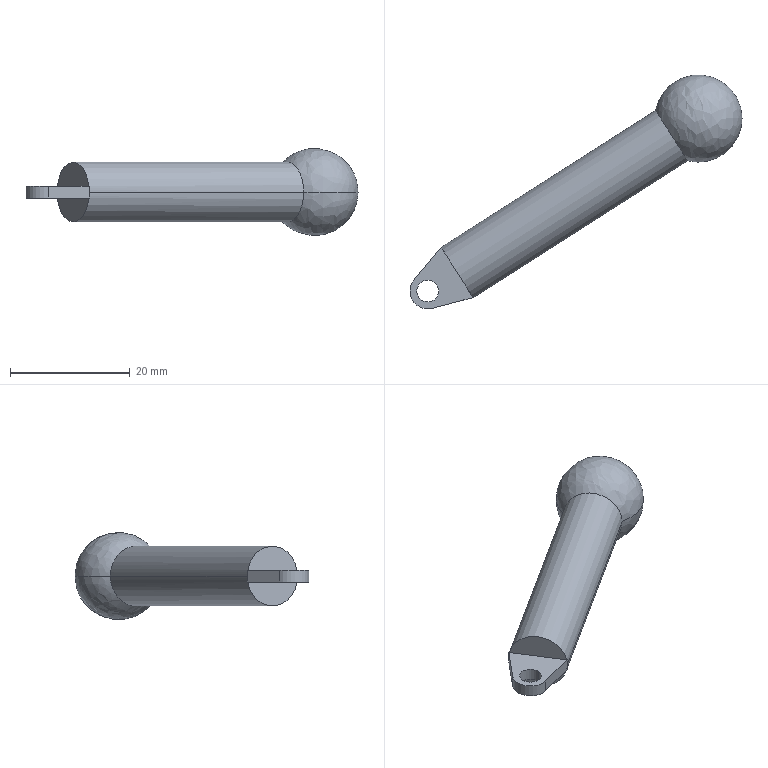Part | SolidWorks | features BaseBody 1 | 1 solid | 17 faces | box 55.474 x 39.094 x 14.478 mm | volume 4963 mm3 | plane 10 | cylinder 5 | spline 2 | commonest cylinder face diameters 3.663 x2 9.977 x2 5.943 x1
STEP:
#1=CARTESIAN_POINT('',(-130.74,-10.361,0.));
#2=VERTEX_POINT('',#1);
#3=CARTESIAN_POINT('',(-145.183,-9.009,0.));
#4=VERTEX_POINT('',#3);
#5=CARTESIAN_POINT('',(-138.024,-10.361,0.));
#6=DIRECTION('',(0.,0.,1.));
#7=DIRECTION('',(1.,0.,0.));
#8=AXIS2_PLACEMENT_3D('',#5,#6,#7);
#9=CIRCLE('',#8,7.285);
#10=EDGE_CURVE('',#2,#4,#9,.T.);
#11=ORIENTED_EDGE('',*,*,#10,.F.);
#12=CARTESIAN_POINT('',(-139.818,-17.421,0.));
#13=VERTEX_POINT('',#12);
#14=CARTESIAN_POINT('',(-138.024,-10.361,0.));
#15=DIRECTION('',(0.,0.,-1.));
#16=DIRECTION('',(1.,0.,0.));
#17=AXIS2_PLACEMENT_3D('',#14,#15,#16);
#18=CIRCLE('',#17,7.285);
#19=EDGE_CURVE('',#2,#13,#18,.T.);
#20=ORIENTED_EDGE('',*,*,#19,.T.);
#21=CARTESIAN_POINT('',(-142.5,-13.215,0.));
#22=DIRECTION('',(-0.8431,-0.5377,0.));
#23=DIRECTION('',(-0.5377,0.8431,0.));
#24=AXIS2_PLACEMENT_3D('',#21,#22,#23);
#25=CIRCLE('',#24,4.989);
#26=EDGE_CURVE('',#4,#13,#25,.T.);
#27=ORIENTED_EDGE('',*,*,#26,.F.);
#28=EDGE_LOOP('',(#11,#20,#27));
#29=FACE_OUTER_BOUND('',#28,.T.);
#30=CARTESIAN_POINT('',(-130.74,-10.361,0.));
#31=CARTESIAN_POINT('',(-130.74,-10.361,0.));
#32=CARTESIAN_POINT('',(-130.74,-10.361,0.));
#33=CARTESIAN_POINT('',(-130.74,-10.361,0.));
#34=CARTESIAN_POINT('',(-130.74,-22.783,0.));
#35=CARTESIAN_POINT('',(-130.74,-22.783,-24.844));
#36=CARTESIAN_POINT('',(-130.74,2.061,-24.844));
#37=CARTESIAN_POINT('',(-130.74,2.061,0.));
#38=CARTESIAN_POINT('',(-143.118,-23.83,0.));
#39=CARTESIAN_POINT('',(-143.118,-23.83,-26.94));
#40=CARTESIAN_POINT('',(-143.118,3.109,-26.94));
#41=CARTESIAN_POINT('',(-143.118,3.109,0.));
#42=CARTESIAN_POINT('',(-145.205,-11.585,0.));
#43=CARTESIAN_POINT('',(-145.205,-11.585,-2.449));
#44=CARTESIAN_POINT('',(-145.205,-9.136,-2.449));
#45=CARTESIAN_POINT('',(-145.205,-9.136,0.));
#46=(BOUNDED_SURFACE()B_SPLINE_SURFACE(3,3,((#30,#31,#32,#33),(#34,#35,#36,#37),(#38,#39,#40,#41),(#42,#43,#44,#45)),.UNSPECIFIED.,.F.,.F.,.F.)B_SPLINE_SURFACE_WITH_KNOTS((4,4),(4,4),(0.,1.),(0.,1.),.UNSPECIFIED.)GEOMETRIC_REPRESENTATION_ITEM()RATIONAL_B_SPLINE_SURFACE(((1.,0.3333,0.3333,1.),(0.3896,0.1299,0.1299,0.3896),(0.3896,0.1299,0.1299,0.3896),(1.,0.3333,0.3333,1.)))REPRESENTATION_ITEM('')SURFACE());
#47=ADVANCED_FACE('',(#29),#46,.T.);
#48=CARTESIAN_POINT('',(-175.716,-40.195,1.));
#49=VERTEX_POINT('',#48);
#50=CARTESIAN_POINT('',(-175.661,-40.281,0.));
#51=VERTEX_POINT('',#50);
#52=CARTESIAN_POINT('',(-178.344,-36.075,0.));
#53=DIRECTION('',(0.8431,0.5377,0.));
#54=DIRECTION('',(-0.5377,0.8431,0.));
#55=AXIS2_PLACEMENT_3D('',#52,#53,#54);
#56=CIRCLE('',#55,4.989);
#57=EDGE_CURVE('',#49,#51,#56,.T.);
#58=ORIENTED_EDGE('',*,*,#57,.T.);
#59=CARTESIAN_POINT('',(-157.74,-28.851,0.));
#60=DIRECTION('',(0.8431,0.5377,0.));
#61=VECTOR('',#60,1000.);
#62=LINE('',#59,#61);
#63=EDGE_CURVE('',#51,#13,#62,.T.);
#64=ORIENTED_EDGE('',*,*,#63,.T.);
#65=CARTESIAN_POINT('',(-142.5,-13.215,0.));
#66=DIRECTION('',(-0.8431,-0.5377,0.));
#67=DIRECTION('',(-0.5377,0.8431,0.));
#68=AXIS2_PLACEMENT_3D('',#65,#66,#67);
#69=CIRCLE('',#68,4.989);
#70=EDGE_CURVE('',#13,#4,#69,.T.);
#71=ORIENTED_EDGE('',*,*,#70,.T.);
#72=CARTESIAN_POINT('',(-181.026,-31.869,0.));
#73=VERTEX_POINT('',#72);
#74=CARTESIAN_POINT('',(-163.104,-20.439,0.));
#75=DIRECTION('',(0.8431,0.5377,0.));
#76=VECTOR('',#75,1000.);
#77=LINE('',#74,#76);
#78=EDGE_CURVE('',#73,#4,#77,.T.);
#79=ORIENTED_EDGE('',*,*,#78,.F.);
#80=CARTESIAN_POINT('',(-180.972,-31.954,1.));
#81=VERTEX_POINT('',#80);
#82=CARTESIAN_POINT('',(-178.344,-36.075,0.));
#83=DIRECTION('',(0.8431,0.5377,0.));
#84=DIRECTION('',(-0.5377,0.8431,0.));
#85=AXIS2_PLACEMENT_3D('',#82,#83,#84);
#86=CIRCLE('',#85,4.989);
#87=EDGE_CURVE('',#73,#81,#86,.T.);
#88=ORIENTED_EDGE('',*,*,#87,.T.);
#89=CARTESIAN_POINT('',(-178.344,-36.075,0.));
#90=DIRECTION('',(0.8431,0.5377,0.));
#91=DIRECTION('',(-0.5377,0.8431,0.));
#92=AXIS2_PLACEMENT_3D('',#89,#90,#91);
#93=CIRCLE('',#92,4.989);
#94=EDGE_CURVE('',#81,#49,#93,.T.);
#95=ORIENTED_EDGE('',*,*,#94,.T.);
#96=EDGE_LOOP('',(#58,#64,#71,#79,#88,#95));
#97=FACE_OUTER_BOUND('',#96,.T.);
#98=CARTESIAN_POINT('',(-160.422,-24.645,0.));
#99=DIRECTION('',(0.8431,0.5377,0.));
#100=DIRECTION('',(-0.5377,0.8431,0.));
#101=AXIS2_PLACEMENT_3D('',#98,#99,#100);
#102=CYLINDRICAL_SURFACE('',#101,4.989);
#103=ADVANCED_FACE('',(#97),#102,.T.);
#104=CARTESIAN_POINT('',(-181.411,-39.199,-1.));
#105=VERTEX_POINT('',#104);
#106=CARTESIAN_POINT('',(-185.074,-39.199,-1.));
#107=VERTEX_POINT('',#106);
#108=CARTESIAN_POINT('',(-183.243,-39.199,-1.));
#109=DIRECTION('',(0.,0.,-1.));
#110=DIRECTION('',(1.,0.,0.));
#111=AXIS2_PLACEMENT_3D('',#108,#109,#110);
#112=CIRCLE('',#111,1.832);
#113=EDGE_CURVE('',#105,#107,#112,.T.);
#114=ORIENTED_EDGE('',*,*,#113,.T.);
#115=CARTESIAN_POINT('',(-185.074,-39.199,1.));
#116=VERTEX_POINT('',#115);
#117=CARTESIAN_POINT('',(-185.074,-39.199,0.));
#118=DIRECTION('',(0.,0.,1.));
#119=VECTOR('',#118,1000.);
#120=LINE('',#117,#119);
#121=EDGE_CURVE('',#107,#116,#120,.T.);
#122=ORIENTED_EDGE('',*,*,#121,.T.);
#123=CARTESIAN_POINT('',(-181.411,-39.199,1.));
#124=VERTEX_POINT('',#123);
#125=CARTESIAN_POINT('',(-183.243,-39.199,1.));
#126=DIRECTION('',(0.,0.,-1.));
#127=DIRECTION('',(1.,0.,0.));
#128=AXIS2_PLACEMENT_3D('',#125,#126,#127);
#129=CIRCLE('',#128,1.832);
#130=EDGE_CURVE('',#124,#116,#129,.T.);
#131=ORIENTED_EDGE('',*,*,#130,.F.);
#132=CARTESIAN_POINT('',(-181.411,-39.199,0.));
#133=DIRECTION('',(0.,0.,1.));
#134=VECTOR('',#133,1000.);
#135=LINE('',#132,#134);
#136=EDGE_CURVE('',#105,#124,#135,.T.);
#137=ORIENTED_EDGE('',*,*,#136,.F.);
#138=EDGE_LOOP('',(#114,#122,#131,#137));
#139=FACE_OUTER_BOUND('',#138,.T.);
#140=CARTESIAN_POINT('',(-183.243,-39.199,0.));
#141=DIRECTION('',(0.,0.,1.));
#142=DIRECTION('',(1.,0.,0.));
#143=AXIS2_PLACEMENT_3D('',#140,#141,#142);
#144=CYLINDRICAL_SURFACE('',#143,1.832);
#145=ADVANCED_FACE('',(#139),#144,.F.);
#146=ORIENTED_EDGE('',*,*,#63,.F.);
#147=CARTESIAN_POINT('',(-175.716,-40.195,-1.));
#148=VERTEX_POINT('',#147);
#149=CARTESIAN_POINT('',(-178.344,-36.075,0.));
#150=DIRECTION('',(0.8431,0.5377,0.));
#151=DIRECTION('',(-0.5377,0.8431,0.));
#152=AXIS2_PLACEMENT_3D('',#149,#150,#151);
#153=CIRCLE('',#152,4.989);
#154=EDGE_CURVE('',#51,#148,#153,.T.);
#155=ORIENTED_EDGE('',*,*,#154,.T.);
#156=CARTESIAN_POINT('',(-180.972,-31.954,-1.));
#157=VERTEX_POINT('',#156);
#158=CARTESIAN_POINT('',(-178.344,-36.075,0.));
#159=DIRECTION('',(0.8431,0.5377,0.));
#160=DIRECTION('',(-0.5377,0.8431,0.));
#161=AXIS2_PLACEMENT_3D('',#158,#159,#160);
#162=CIRCLE('',#161,4.989);
#163=EDGE_CURVE('',#148,#157,#162,.T.);
#164=ORIENTED_EDGE('',*,*,#163,.T.);
#165=CARTESIAN_POINT('',(-178.344,-36.075,0.));
#166=DIRECTION('',(0.8431,0.5377,0.));
#167=DIRECTION('',(-0.5377,0.8431,0.));
#168=AXIS2_PLACEMENT_3D('',#165,#166,#167);
#169=CIRCLE('',#168,4.989);
#170=EDGE_CURVE('',#157,#73,#169,.T.);
#171=ORIENTED_EDGE('',*,*,#170,.T.);
#172=ORIENTED_EDGE('',*,*,#78,.T.);
#173=ORIENTED_EDGE('',*,*,#26,.T.);
#174=EDGE_LOOP('',(#146,#155,#164,#171,#172,#173));
#175=FACE_OUTER_BOUND('',#174,.T.);
#176=CARTESIAN_POINT('',(-160.422,-24.645,0.));
#177=DIRECTION('',(0.8431,0.5377,0.));
#178=DIRECTION('',(-0.5377,0.8431,0.));
#179=AXIS2_PLACEMENT_3D('',#176,#177,#178);
#180=CYLINDRICAL_SURFACE('',#179,4.989);
#181=ADVANCED_FACE('',(#175),#180,.T.);
#182=ORIENTED_EDGE('',*,*,#19,.F.);
#183=ORIENTED_EDGE('',*,*,#10,.T.);
#184=ORIENTED_EDGE('',*,*,#70,.F.);
#185=EDGE_LOOP('',(#182,#183,#184));
#186=FACE_OUTER_BOUND('',#185,.T.);
#187=CARTESIAN_POINT('',(-130.74,-10.361,0.));
#188=CARTESIAN_POINT('',(-130.74,-10.361,0.));
#189=CARTESIAN_POINT('',(-130.74,-10.361,0.));
#190=CARTESIAN_POINT('',(-130.74,-10.361,0.));
#191=CARTESIAN_POINT('',(-130.74,2.061,0.));
#192=CARTESIAN_POINT('',(-130.74,2.061,24.844));
#193=CARTESIAN_POINT('',(-130.74,-22.783,24.844));
#194=CARTESIAN_POINT('',(-130.74,-22.783,0.));
#195=CARTESIAN_POINT('',(-143.118,3.109,0.));
#196=CARTESIAN_POINT('',(-143.118,3.109,26.94));
#197=CARTESIAN_POINT('',(-143.118,-23.83,26.94));
#198=CARTESIAN_POINT('',(-143.118,-23.83,0.));
#199=CARTESIAN_POINT('',(-145.205,-9.136,0.));
#200=CARTESIAN_POINT('',(-145.205,-9.136,2.449));
#201=CARTESIAN_POINT('',(-145.205,-11.585,2.449));
#202=CARTESIAN_POINT('',(-145.205,-11.585,0.));
#203=(BOUNDED_SURFACE()B_SPLINE_SURFACE(3,3,((#187,#188,#189,#190),(#191,#192,#193,#194),(#195,#196,#197,#198),(#199,#200,#201,#202)),.UNSPECIFIED.,.F.,.F.,.F.)B_SPLINE_SURFACE_WITH_KNOTS((4,4),(4,4),(0.,1.),(0.,1.),.UNSPECIFIED.)GEOMETRIC_REPRESENTATION_ITEM()RATIONAL_B_SPLINE_SURFACE(((1.,0.3333,0.3333,1.),(0.3896,0.1299,0.1299,0.3896),(0.3896,0.1299,0.1299,0.3896),(1.,0.3333,0.3333,1.)))REPRESENTATION_ITEM('')SURFACE());
#204=ADVANCED_FACE('',(#186),#203,.T.);
#205=CARTESIAN_POINT('',(-175.661,-40.281,1.));
#206=VERTEX_POINT('',#205);
#207=CARTESIAN_POINT('',(-175.661,-40.281,1.));
#208=DIRECTION('',(-0.5377,0.8431,0.));
#209=VECTOR('',#208,1000.);
#210=LINE('',#207,#209);
#211=EDGE_CURVE('',#206,#49,#210,.T.);
#212=ORIENTED_EDGE('',*,*,#211,.F.);
#213=CARTESIAN_POINT('',(-175.661,-40.281,0.));
#214=DIRECTION('',(0.,0.,1.));
#215=VECTOR('',#214,1000.);
#216=LINE('',#213,#215);
#217=EDGE_CURVE('',#51,#206,#216,.T.);
#218=ORIENTED_EDGE('',*,*,#217,.F.);
#219=ORIENTED_EDGE('',*,*,#57,.F.);
#220=EDGE_LOOP('',(#212,#218,#219));
#221=FACE_OUTER_BOUND('',#220,.T.);
#222=CARTESIAN_POINT('',(-175.661,-40.281,0.));
#223=DIRECTION('',(0.8431,0.5377,0.));
#224=DIRECTION('',(-0.5377,0.8431,0.));
#225=AXIS2_PLACEMENT_3D('',#222,#223,#224);
#226=PLANE('',#225);
#227=ADVANCED_FACE('',(#221),#226,.T.);
#228=CARTESIAN_POINT('',(-181.026,-31.869,1.));
#229=DIRECTION('',(0.5377,-0.8431,0.));
#230=VECTOR('',#229,1000.);
#231=LINE('',#228,#230);
#232=EDGE_CURVE('',#81,#49,#231,.T.);
#233=ORIENTED_EDGE('',*,*,#232,.T.);
#234=ORIENTED_EDGE('',*,*,#94,.F.);
#235=EDGE_LOOP('',(#233,#234));
#236=FACE_OUTER_BOUND('',#235,.T.);
#237=CARTESIAN_POINT('',(-181.026,-31.869,0.));
#238=DIRECTION('',(-0.8431,-0.5377,0.));
#239=DIRECTION('',(0.5377,-0.8431,0.));
#240=AXIS2_PLACEMENT_3D('',#237,#238,#239);
#241=PLANE('',#240);
#242=ADVANCED_FACE('',(#236),#241,.T.);
#243=CARTESIAN_POINT('',(-181.026,-31.869,1.));
#244=VERTEX_POINT('',#243);
#245=CARTESIAN_POINT('',(-181.026,-31.869,0.));
#246=DIRECTION('',(0.,0.,-1.));
#247=VECTOR('',#246,1000.);
#248=LINE('',#245,#247);
#249=EDGE_CURVE('',#244,#73,#248,.T.);
#250=ORIENTED_EDGE('',*,*,#249,.F.);
#251=CARTESIAN_POINT('',(-175.661,-40.281,1.));
#252=DIRECTION('',(0.5377,-0.8431,0.));
#253=VECTOR('',#252,1000.);
#254=LINE('',#251,#253);
#255=EDGE_CURVE('',#244,#81,#254,.T.);
#256=ORIENTED_EDGE('',*,*,#255,.T.);
#257=ORIENTED_EDGE('',*,*,#87,.F.);
#258=EDGE_LOOP('',(#250,#256,#257));
#259=FACE_OUTER_BOUND('',#258,.T.);
#260=CARTESIAN_POINT('',(-175.661,-40.281,0.));
#261=DIRECTION('',(0.8431,0.5377,0.));
#262=DIRECTION('',(-0.5377,0.8431,0.));
#263=AXIS2_PLACEMENT_3D('',#260,#261,#262);
#264=PLANE('',#263);
#265=ADVANCED_FACE('',(#259),#264,.T.);
#266=CARTESIAN_POINT('',(-181.026,-31.869,-1.));
#267=VERTEX_POINT('',#266);
#268=CARTESIAN_POINT('',(-180.972,-31.954,-1.));
#269=DIRECTION('',(-0.5377,0.8431,0.));
#270=VECTOR('',#269,1000.);
#271=LINE('',#268,#270);
#272=EDGE_CURVE('',#157,#267,#271,.T.);
#273=ORIENTED_EDGE('',*,*,#272,.T.);
#274=CARTESIAN_POINT('',(-181.026,-31.869,0.));
#275=DIRECTION('',(0.,0.,-1.));
#276=VECTOR('',#275,1000.);
#277=LINE('',#274,#276);
#278=EDGE_CURVE('',#73,#267,#277,.T.);
#279=ORIENTED_EDGE('',*,*,#278,.F.);
#280=ORIENTED_EDGE('',*,*,#170,.F.);
#281=EDGE_LOOP('',(#273,#279,#280));
#282=FACE_OUTER_BOUND('',#281,.T.);
#283=CARTESIAN_POINT('',(-175.661,-40.281,0.));
#284=DIRECTION('',(0.8431,0.5377,0.));
#285=DIRECTION('',(-0.5377,0.8431,0.));
#286=AXIS2_PLACEMENT_3D('',#283,#284,#285);
#287=PLANE('',#286);
#288=ADVANCED_FACE('',(#282),#287,.T.);
#289=CARTESIAN_POINT('',(-181.026,-31.869,-1.));
#290=DIRECTION('',(-0.5377,0.8431,0.));
#291=VECTOR('',#290,1000.);
#292=LINE('',#289,#291);
#293=EDGE_CURVE('',#148,#157,#292,.T.);
#294=ORIENTED_EDGE('',*,*,#293,.T.);
#295=ORIENTED_EDGE('',*,*,#163,.F.);
#296=EDGE_LOOP('',(#294,#295));
#297=FACE_OUTER_BOUND('',#296,.T.);
#298=CARTESIAN_POINT('',(-181.026,-31.869,0.));
#299=DIRECTION('',(-0.8431,-0.5377,0.));
#300=DIRECTION('',(0.5377,-0.8431,0.));
#301=AXIS2_PLACEMENT_3D('',#298,#299,#300);
#302=PLANE('',#301);
#303=ADVANCED_FACE('',(#297),#302,.T.);
#304=CARTESIAN_POINT('',(-175.661,-40.281,-1.));
#305=VERTEX_POINT('',#304);
#306=CARTESIAN_POINT('',(-175.661,-40.281,0.));
#307=DIRECTION('',(0.,0.,1.));
#308=VECTOR('',#307,1000.);
#309=LINE('',#306,#308);
#310=EDGE_CURVE('',#305,#51,#309,.T.);
#311=ORIENTED_EDGE('',*,*,#310,.F.);
#312=CARTESIAN_POINT('',(-175.661,-40.281,-1.));
#313=DIRECTION('',(-0.5377,0.8431,0.));
#314=VECTOR('',#313,1000.);
#315=LINE('',#312,#314);
#316=EDGE_CURVE('',#305,#148,#315,.T.);
#317=ORIENTED_EDGE('',*,*,#316,.T.);
#318=ORIENTED_EDGE('',*,*,#154,.F.);
#319=EDGE_LOOP('',(#311,#317,#318));
#320=FACE_OUTER_BOUND('',#319,.T.);
#321=CARTESIAN_POINT('',(-175.661,-40.281,0.));
#322=DIRECTION('',(0.8431,0.5377,0.));
#323=DIRECTION('',(-0.5377,0.8431,0.));
#324=AXIS2_PLACEMENT_3D('',#321,#322,#323);
#325=PLANE('',#324);
#326=ADVANCED_FACE('',(#320),#325,.T.);
#327=ORIENTED_EDGE('',*,*,#130,.T.);
#328=CARTESIAN_POINT('',(-183.243,-39.199,1.));
#329=DIRECTION('',(0.,0.,-1.));
#330=DIRECTION('',(1.,0.,0.));
#331=AXIS2_PLACEMENT_3D('',#328,#329,#330);
#332=CIRCLE('',#331,1.832);
#333=EDGE_CURVE('',#116,#124,#332,.T.);
#334=ORIENTED_EDGE('',*,*,#333,.T.);
#335=EDGE_LOOP('',(#327,#334));
#336=FACE_BOUND('',#335,.T.);
#337=ORIENTED_EDGE('',*,*,#232,.F.);
#338=ORIENTED_EDGE('',*,*,#255,.F.);
#339=CARTESIAN_POINT('',(-185.53,-37.303,1.));
#340=VERTEX_POINT('',#339);
#341=CARTESIAN_POINT('',(-181.026,-31.869,1.));
#342=DIRECTION('',(-0.6382,-0.7699,0.));
#343=VECTOR('',#342,1000.);
#344=LINE('',#341,#343);
#345=EDGE_CURVE('',#244,#340,#344,.T.);
#346=ORIENTED_EDGE('',*,*,#345,.T.);
#347=CARTESIAN_POINT('',(-182.488,-42.073,1.));
#348=VERTEX_POINT('',#347);
#349=CARTESIAN_POINT('',(-183.243,-39.199,1.));
#350=DIRECTION('',(0.,0.,1.));
#351=DIRECTION('',(1.,0.,0.));
#352=AXIS2_PLACEMENT_3D('',#349,#350,#351);
#353=CIRCLE('',#352,2.971);
#354=EDGE_CURVE('',#340,#348,#353,.T.);
#355=ORIENTED_EDGE('',*,*,#354,.T.);
#356=CARTESIAN_POINT('',(-182.488,-42.073,1.));
#357=DIRECTION('',(0.9672,0.2539,0.));
#358=VECTOR('',#357,1000.);
#359=LINE('',#356,#358);
#360=EDGE_CURVE('',#348,#206,#359,.T.);
#361=ORIENTED_EDGE('',*,*,#360,.T.);
#362=ORIENTED_EDGE('',*,*,#211,.T.);
#363=EDGE_LOOP('',(#337,#338,#346,#355,#361,#362));
#364=FACE_OUTER_BOUND('',#363,.T.);
#365=CARTESIAN_POINT('',(-180.938,-37.02,1.));
#366=DIRECTION('',(0.,0.,1.));
#367=DIRECTION('',(1.,0.,0.));
#368=AXIS2_PLACEMENT_3D('',#365,#366,#367);
#369=PLANE('',#368);
#370=ADVANCED_FACE('',(#336,#364),#369,.T.);
#371=ORIENTED_EDGE('',*,*,#113,.F.);
#372=CARTESIAN_POINT('',(-183.243,-39.199,-1.));
#373=DIRECTION('',(0.,0.,-1.));
#374=DIRECTION('',(1.,0.,0.));
#375=AXIS2_PLACEMENT_3D('',#372,#373,#374);
#376=CIRCLE('',#375,1.832);
#377=EDGE_CURVE('',#107,#105,#376,.T.);
#378=ORIENTED_EDGE('',*,*,#377,.F.);
#379=EDGE_LOOP('',(#371,#378));
#380=FACE_BOUND('',#379,.T.);
#381=ORIENTED_EDGE('',*,*,#272,.F.);
#382=ORIENTED_EDGE('',*,*,#293,.F.);
#383=ORIENTED_EDGE('',*,*,#316,.F.);
#384=CARTESIAN_POINT('',(-182.488,-42.073,-1.));
#385=VERTEX_POINT('',#384);
#386=CARTESIAN_POINT('',(-182.488,-42.073,-1.));
#387=DIRECTION('',(0.9672,0.2539,0.));
#388=VECTOR('',#387,1000.);
#389=LINE('',#386,#388);
#390=EDGE_CURVE('',#385,#305,#389,.T.);
#391=ORIENTED_EDGE('',*,*,#390,.F.);
#392=CARTESIAN_POINT('',(-185.53,-37.303,-1.));
#393=VERTEX_POINT('',#392);
#394=CARTESIAN_POINT('',(-183.243,-39.199,-1.));
#395=DIRECTION('',(0.,0.,1.));
#396=DIRECTION('',(1.,0.,0.));
#397=AXIS2_PLACEMENT_3D('',#394,#395,#396);
#398=CIRCLE('',#397,2.971);
#399=EDGE_CURVE('',#393,#385,#398,.T.);
#400=ORIENTED_EDGE('',*,*,#399,.F.);
#401=CARTESIAN_POINT('',(-181.026,-31.869,-1.));
#402=DIRECTION('',(-0.6382,-0.7699,0.));
#403=VECTOR('',#402,1000.);
#404=LINE('',#401,#403);
#405=EDGE_CURVE('',#267,#393,#404,.T.);
#406=ORIENTED_EDGE('',*,*,#405,.F.);
#407=EDGE_LOOP('',(#381,#382,#383,#391,#400,#406));
#408=FACE_OUTER_BOUND('',#407,.T.);
#409=CARTESIAN_POINT('',(-180.938,-37.02,-1.));
#410=DIRECTION('',(0.,0.,1.));
#411=DIRECTION('',(1.,0.,0.));
#412=AXIS2_PLACEMENT_3D('',#409,#410,#411);
#413=PLANE('',#412);
#414=ADVANCED_FACE('',(#380,#408),#413,.F.);
#415=ORIENTED_EDGE('',*,*,#121,.F.);
#416=ORIENTED_EDGE('',*,*,#377,.T.);
#417=ORIENTED_EDGE('',*,*,#136,.T.);
#418=ORIENTED_EDGE('',*,*,#333,.F.);
#419=EDGE_LOOP('',(#415,#416,#417,#418));
#420=FACE_OUTER_BOUND('',#419,.T.);
#421=CARTESIAN_POINT('',(-183.243,-39.199,0.));
#422=DIRECTION('',(0.,0.,1.));
#423=DIRECTION('',(1.,0.,0.));
#424=AXIS2_PLACEMENT_3D('',#421,#422,#423);
#425=CYLINDRICAL_SURFACE('',#424,1.832);
#426=ADVANCED_FACE('',(#420),#425,.F.);
#427=CARTESIAN_POINT('',(-182.488,-42.073,0.));
#428=DIRECTION('',(0.,0.,-1.));
#429=VECTOR('',#428,1000.);
#430=LINE('',#427,#429);
#431=EDGE_CURVE('',#348,#385,#430,.T.);
#432=ORIENTED_EDGE('',*,*,#431,.T.);
#433=ORIENTED_EDGE('',*,*,#390,.T.);
#434=ORIENTED_EDGE('',*,*,#310,.T.);
#435=ORIENTED_EDGE('',*,*,#217,.T.);
#436=ORIENTED_EDGE('',*,*,#360,.F.);
#437=EDGE_LOOP('',(#432,#433,#434,#435,#436));
#438=FACE_OUTER_BOUND('',#437,.T.);
#439=CARTESIAN_POINT('',(-182.488,-42.073,0.));
#440=DIRECTION('',(0.2539,-0.9672,0.));
#441=DIRECTION('',(0.9672,0.2539,0.));
#442=AXIS2_PLACEMENT_3D('',#439,#440,#441);
#443=PLANE('',#442);
#444=ADVANCED_FACE('',(#438),#443,.T.);
#445=CARTESIAN_POINT('',(-185.53,-37.303,0.));
#446=DIRECTION('',(0.,0.,-1.));
#447=VECTOR('',#446,1000.);
#448=LINE('',#445,#447);
#449=EDGE_CURVE('',#340,#393,#448,.T.);
#450=ORIENTED_EDGE('',*,*,#449,.T.);
#451=ORIENTED_EDGE('',*,*,#399,.T.);
#452=ORIENTED_EDGE('',*,*,#431,.F.);
#453=ORIENTED_EDGE('',*,*,#354,.F.);
#454=EDGE_LOOP('',(#450,#451,#452,#453));
#455=FACE_OUTER_BOUND('',#454,.T.);
#456=CARTESIAN_POINT('',(-183.243,-39.199,0.));
#457=DIRECTION('',(0.,0.,1.));
#458=DIRECTION('',(1.,0.,0.));
#459=AXIS2_PLACEMENT_3D('',#456,#457,#458);
#460=CYLINDRICAL_SURFACE('',#459,2.971);
#461=ADVANCED_FACE('',(#455),#460,.T.);
#462=ORIENTED_EDGE('',*,*,#278,.T.);
#463=ORIENTED_EDGE('',*,*,#405,.T.);
#464=ORIENTED_EDGE('',*,*,#449,.F.);
#465=ORIENTED_EDGE('',*,*,#345,.F.);
#466=ORIENTED_EDGE('',*,*,#249,.T.);
#467=EDGE_LOOP('',(#462,#463,#464,#465,#466));
#468=FACE_OUTER_BOUND('',#467,.T.);
#469=CARTESIAN_POINT('',(-181.026,-31.869,0.));
#470=DIRECTION('',(-0.7699,0.6382,0.));
#471=DIRECTION('',(-0.6382,-0.7699,0.));
#472=AXIS2_PLACEMENT_3D('',#469,#470,#471);
#473=PLANE('',#472);
#474=ADVANCED_FACE('',(#468),#473,.T.);
#475=CLOSED_SHELL('',(#47,#103,#145,#181,#204,#227,#242,#265,#288,#303,#326,#370,#414,#426,#444,#461,#474));
#476=MANIFOLD_SOLID_BREP('',#475);
#477=CARTESIAN_POINT('',(0.,0.,0.));
#478=DIRECTION('',(0.,0.,1.));
#479=DIRECTION('',(1.,0.,0.));
#480=AXIS2_PLACEMENT_3D('',#477,#478,#479);
#481=(LENGTH_UNIT()NAMED_UNIT(*)SI_UNIT(.MILLI.,.METRE.));
#482=UNCERTAINTY_MEASURE_WITH_UNIT(LENGTH_MEASURE(0.00001),#481,'','');
#483=(NAMED_UNIT(*)PLANE_ANGLE_UNIT()SI_UNIT($,.RADIAN.));
#484=(NAMED_UNIT(*)SI_UNIT($,.STERADIAN.)SOLID_ANGLE_UNIT());
#485=(GEOMETRIC_REPRESENTATION_CONTEXT(3)GLOBAL_UNCERTAINTY_ASSIGNED_CONTEXT((#482))GLOBAL_UNIT_ASSIGNED_CONTEXT((#481,#483,#484))REPRESENTATION_CONTEXT('',''));
#486=ADVANCED_BREP_SHAPE_REPRESENTATION('',(#476,#480),#485);